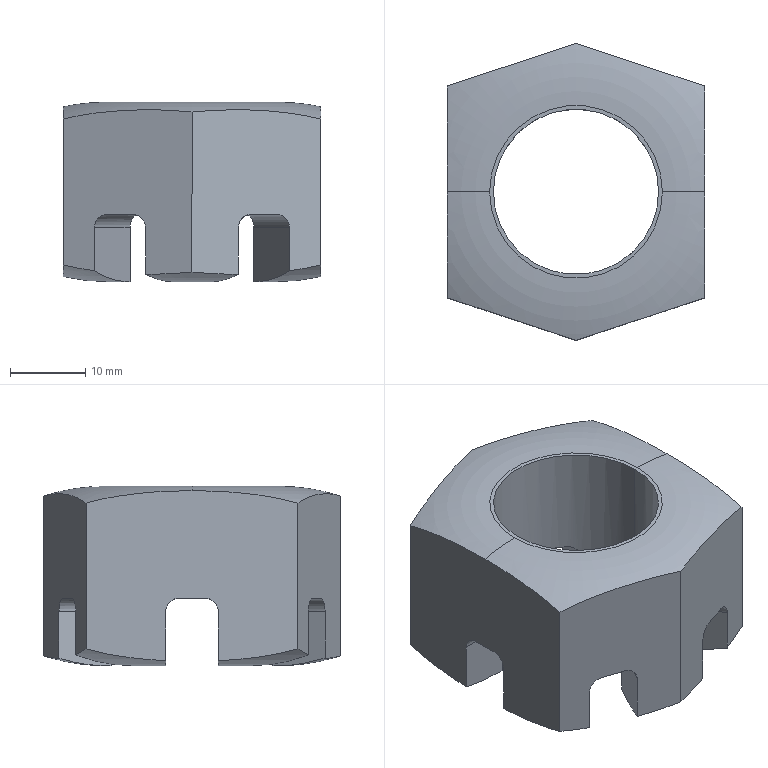Part | SolidWorks | features CirPattern 1, Extrusion 1, Fillet 1, HoleWzd 1, ICE 1, RefAxis 1, RevCut 1 | 1 solid | 53 faces | box 34.3 x 39.5 x 23.9 mm | volume 15247 mm3 | plane 31 | cylinder 14 | torus 8 | commonest cylinder face diameters 3.6 x12 22 x2